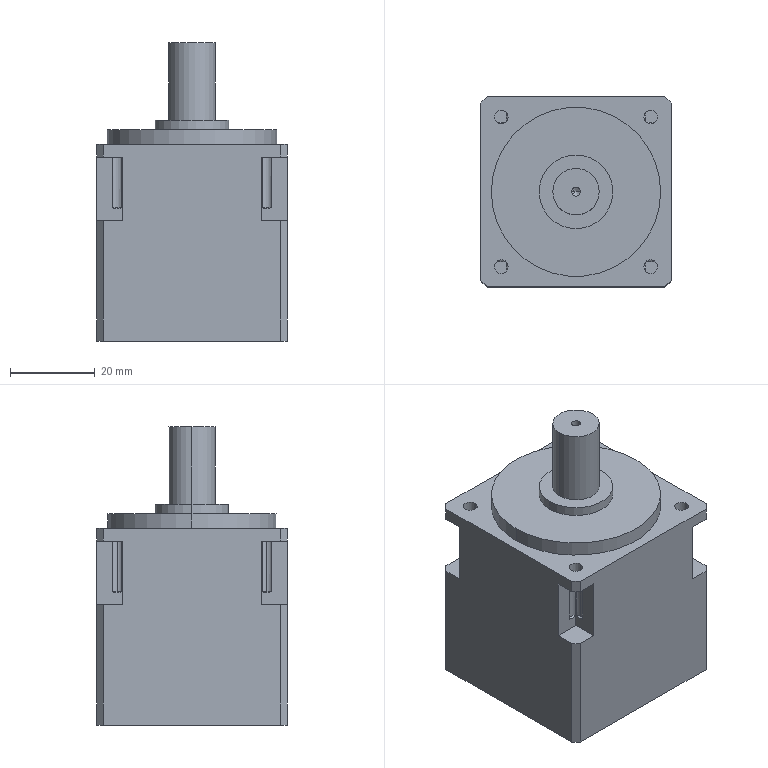Part | SolidWorks | features BaseBody 1, Scale 1 | 1 solid | 64 faces | box 45 x 45 x 70.5 mm | volume 98334 mm3 | plane 37 | cylinder 16 | cone 11 | commonest cylinder face diameters 3.25 x8 2.1 x2 11 x2 17.45 x2 40 x2